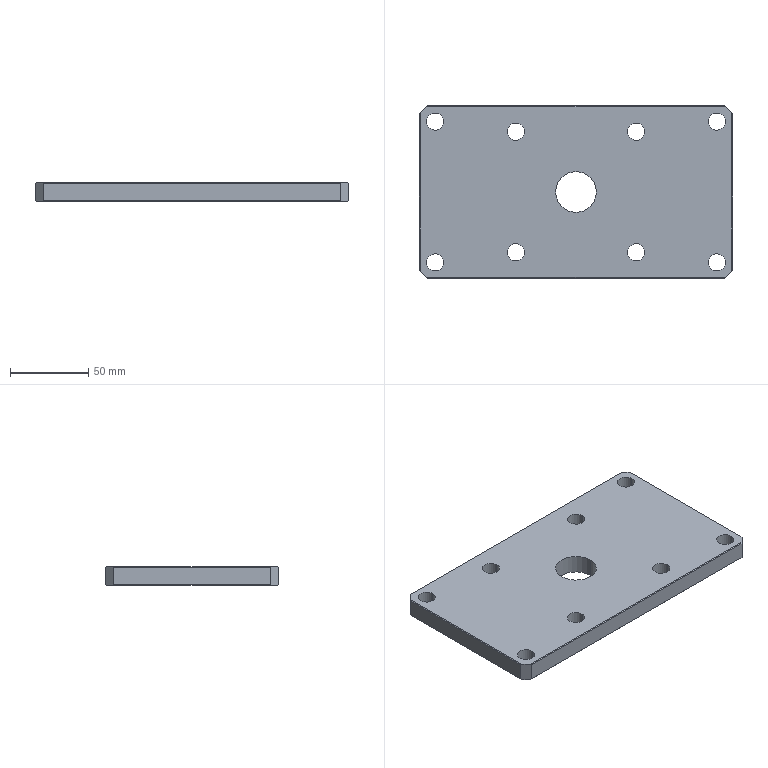Part | STEP file | Large cylinder base plate | 1 solid | 36 faces | box 200 x 110 x 12 mm | volume 247760 mm3 | cylinder 18 | plane 18 | commonest cylinder face diameters 11 x16 26 x2